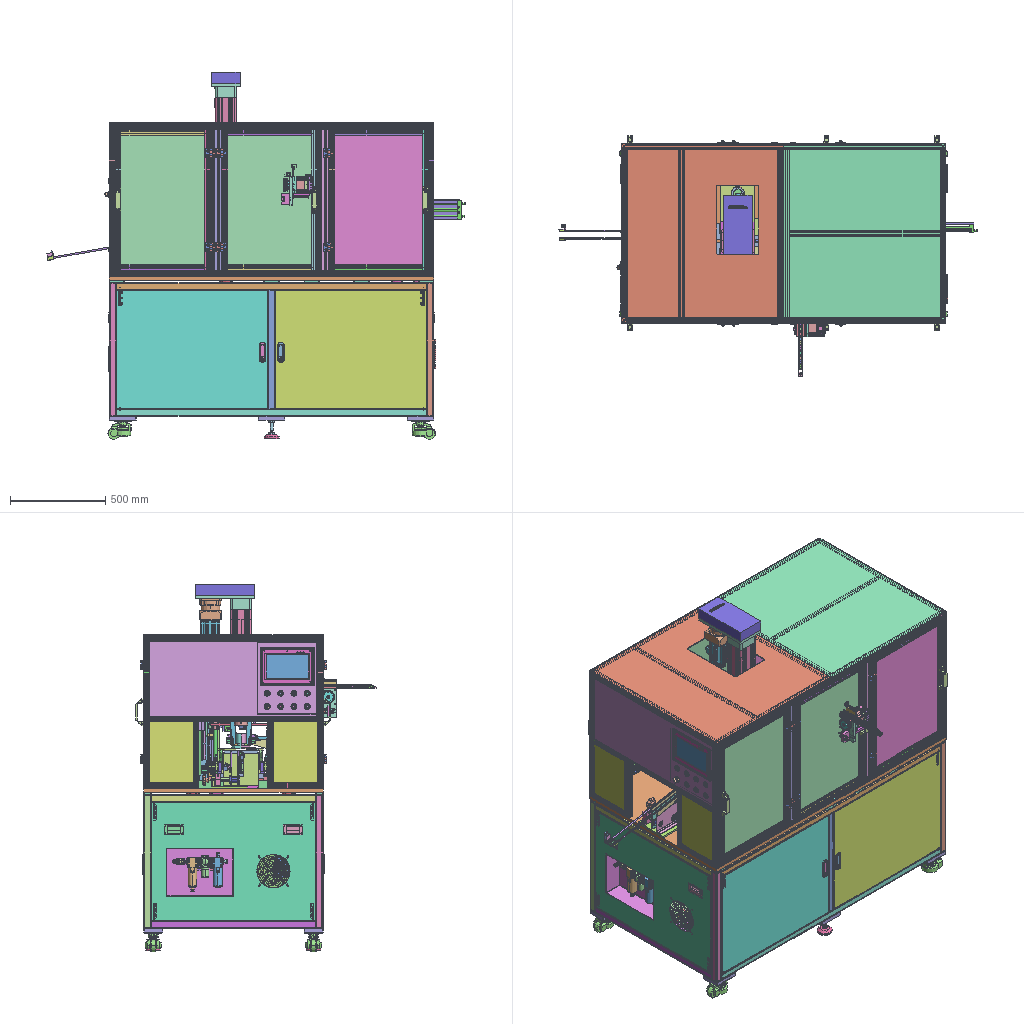Assembly | STEP file | 346 different items | 604 placed | box 2191 x 1257 x 1923 mm
Parts list (item | name | quantity | parent item | size | volume), first 266 of 346 items:
1 | 001-001-Profile frame_default<machined> | x1 | in 001-001-Machine frame_MV-FW80D | 1700 x 940 x 700 mm | 7004652 mm3
2 | 001-001-Small mounting plate | x10 | in 001-001-Machine frame_MV-FW80D | 80 x 40 x 12 mm | 38184 mm3
3 | 001-001-Main load plate | x1 | in 001-001-Machine frame_MV-FW80D | 1700 x 940 x 20 mm | 31960000 mm3
4 | 001-001-Foma caster mounting plate | x6 | in 001-001-Machine frame_MV-FW80D | 140 x 100 x 20 mm | 279640 mm3
5 | 001-001-hcaaa-d80-nj | x4 | in 001-001-Machine frame_MV-FW80D | 90 x 102 x 122.5 mm | 382378 mm3
6 | - | x2 | in 001-001-Machine frame_MV-FW80D | 78 x 134 x 78 mm | 111485 mm3
7 | 001-001-Machine frame door panel | x1 | in 001-001-Machine frame_MV-FW80D | 795 x 624 x 20 mm | 869592 mm3
8 | 001-001-hfy44-96-r | x1 | in 001-001-Machine frame_MV-FW80D | 18 x 22 x 96 mm | 10397 mm3
9 | 001-001-Fixed pin | x1 | in 001-001-Machine frame_MV-FW80D | 8 x 8 x 14 mm | 439.823 mm3
10 | 001-001-xax22-a106 | x1 | in 001-001-Machine frame_MV-FW80D | 69.5 x 40 x 106 mm | 52020 mm3
11 | 001-001- Mirror xax22-a106 | x2 | in 001-001-Machine frame_MV-FW80D | 69.5 x 40 x 106 mm | 52020 mm3
12 | 001-001-Mirror door panel | x2 | in 001-001-Machine frame_MV-FW80D | 795 x 624 x 20 mm | 869592 mm3
13 | 001-001-Mirror fixed pin | x2 | in 001-001-Machine frame_MV-FW80D | 8 x 8 x 14 mm | 439.823 mm3
14 | 001-001- Mirror hfy44-96-r | x3 | in 001-001-Machine frame_MV-FW80D | 18 x 22 x 96 mm | 10397 mm3
15 | 001-001- Mirror Mirror xax22-a106 | x1 | in 001-001-Machine frame_MV-FW80D | 69.5 x 40 x 106 mm | 52020 mm3
16 | 001-001-Mirror Mirror door panel | x1 | in 001-001-Machine frame_MV-FW80D | 795 x 624 x 20 mm | 869592 mm3
17 | 001-001-Mirror Mirror fixed pin | x1 | in 001-001-Machine frame_MV-FW80D | 8 x 8 x 14 mm | 439.823 mm3
18 | 001-001- Mirror Mirror hfy44-96-r | x3 | in 001-001-Machine frame_MV-FW80D | 18 x 22 x 96 mm | 10397 mm3
19 | 001-001-Machine frame end plate | x1 | in 001-001-Machine frame_MV-FW80D | 618 x 858 x 20 mm | 819319 mm3
20 | 001-001- Mirror Mirror Mirror hfy44-96-r | x1 | in 001-001-Machine frame_MV-FW80D | 18 x 22 x 96 mm | 10397 mm3
21 | 001-001-xad51-a100 | x1 | in 001-001-Machine frame_MV-FW80D | 54 x 20.5 x 100 mm | 9020 mm3
22 | 001-001- Mirror xad51-a100 | x1 | in 001-001-Machine frame_MV-FW80D | 54 x 20.5 x 100 mm | 9020 mm3
23 | FKL6622 cabinet fan and filter[FKL6622.230]_filter | x1 | in 001-001-FKL6622 cabinet fan and filter[FKL6622.230]_FKL6622.230 | 24.5 x 148.5 x 148.5 mm | 148645 mm3
24 | FKL6622 cabinet fan and filter[FKL6622.230]_120_G8025HA1S | x1 | in 001-001-FKL6622 cabinet fan and filter[FKL6622.230]_FKL6622.230 | 42.957 x 119.523 x 119.5 mm | 164726 mm3
25 | FKL6622 cabinet fan and filter[FKL6622.230]_TX120 | x1 | in 001-001-FKL6622 cabinet fan and filter[FKL6622.230]_FKL6622.230 | 116 x 5 x 116 mm | 5033 mm3
26 | 001-001-Mirror FKL6622 cabinet fan and filter[FKL6622.230]_filter | x1 | in 001-001-Mirror FKL6622 cabinet fan and filter[FKL6622.230] | 24.5 x 148.5 x 148.5 mm | 148645 mm3
27 | 001-001-Mirror FKL6622 cabinet fan and filter[FKL6622.230]_120_G8025HA1S | x1 | in 001-001-Mirror FKL6622 cabinet fan and filter[FKL6622.230] | 42.957 x 119.523 x 119.5 mm | 164726 mm3
28 | 001-001-Mirror FKL6622 cabinet fan and filter[FKL6622.230]_TX120 | x1 | in 001-001-Mirror FKL6622 cabinet fan and filter[FKL6622.230] | 116 x 5 x 116 mm | 5033 mm3
29 | - | x1 | in 001-001-Machine frame_MV-FW80D | 101.5 x 858 x 618 mm | 647667 mm3
30 | 001-001-Mirror Mirror Mirror hfy44-96-r | x2 | in 001-001-Machine frame_MV-FW80D | 18 x 22 x 96 mm | 10397 mm3
31 | 001-001-Mirrorxad51-a100 | x1 | in 001-001-Machine frame_MV-FW80D | 54 x 20.5 x 100 mm | 9020 mm3
32 | 001-001-Mirror Mirror hfy44-96-r | x1 | in 001-001-Machine frame_MV-FW80D | 18 x 22 x 96 mm | 10397 mm3
33 | 001-001-Mirror Mirror xad51-a100 | x1 | in 001-001-Machine frame_MV-FW80D | 54 x 20.5 x 100 mm | 9020 mm3
34 | 001-001-Mirror Mirror Mirror Mirror hfy44-96-r | x1 | in 001-001-Machine frame_MV-FW80D | 18 x 22 x 96 mm | 10397 mm3
35 | PH1002 | x1 | in 001-001-Air source treatment unit | 39.583 x 28.95 x 18 mm | 7378 mm3
36 | POC1002D | x1 | in 001-001-Air source treatment unit | 17 x 29 x 17 mm | 3444 mm3
37 | GAC30008S | x1 | in 001-001-Air source treatment unit | 195 x 203 x 83 mm | 926577 mm3
38 | HSV10 | x1 | in 001-001-Air source treatment unit | 35.5 x 35.5 x 68.5 mm | 34572 mm3
39 | 001-001-TX180 metal mesh cover[TX180]_TX180 | x1 | in 001-001-Machine frame_MV-FW80D | 175 x 5 x 175 mm | 9660 mm3
40 | 001-001-Machine frame bottom end plate | x2 | in 001-001-Machine frame_MV-FW80D | 788 x 858 x 20 mm | 1465006 mm3
41 | 200M10F | x1 | in 001-001-Valve island assembly | 60 x 24 x 251 mm | 220030 mm3
42 | BSL02 | x3 | in 001-001-Valve island assembly | 17.321 x 30 x 15 mm | 3652 mm3
43 | PC802 | x3 | in 001-001-Valve island assembly | 16.166 x 27 x 14 mm | 2706 mm3
44 | 4V21006B | x10 | in 001-001-Valve island assembly | 22 x 66.8 x 117.8 mm | 101337 mm3
45 | 001-003-Storage mechanism base plate | x1 | in 001-003-Shaft storage mechanism | 370 x 250 x 20 mm | 1842340 mm3
46 | 001-003-Storage mechanism vertical plate | x1 | in 001-003-Shaft storage mechanism | 250 x 550 x 15 mm | 1550347 mm3
47 | 001-003-Storage mechanism rib plate | x2 | in 001-003-Shaft storage mechanism | 110 x 546 x 15 mm | 610650 mm3
48 | - | x1 | - | 20 x 20 x 472 mm | 136774 mm3
49 | - | x1 | - | 44 x 58 x 42 mm | 39340 mm3
50 | 001-003-BK15 | x1 | in 001-003-Shaft storage mechanism | 70 x 48 x 39 mm | 76186 mm3
51 | 001-003-BF15 | x1 | in 001-003-Shaft storage mechanism | 70 x 48 x 20 mm | 44239 mm3
52 | 001-003-Shaft retaining ring 15-1 | x1 | in 001-003-Shaft storage mechanism | 16.7 x 18.72 x 1 mm | 79.464 mm3
53 | 001-003-Shaft storage motor mounting plate | x1 | in 001-003-Shaft storage mechanism | 210 x 71 x 15 mm | 181898 mm3
54 | 001-003-MSMF042L1D2 | x1 | in 001-003-Shaft storage mechanism | 165.5 x 143.937 x 60 mm | 465510 mm3
55 | 001-003-C-SCPS46-12-14 | x1 | in 001-003-Shaft storage mechanism | 29.8 x 46 x 46 mm | 36563 mm3
56 | - | x2 | - | 48 x 34.4 x 96 mm | 105086 mm3
57 | - | x2 | - | 23 x 22 x 480 mm | 205813 mm3
58 | 001-003-Shaft storage slider connecting plate | x1 | in 001-003-Shaft storage mechanism | 250 x 90 x 15 mm | 298680 mm3
59 | 001-003-Shaft storage magazine support plate | x1 | in 001-003-Shaft storage mechanism | 250 x 326 x 15 mm | 922956 mm3
60 | 001-003-Shaft storage magazine rib plate | x2 | in 001-003-Shaft storage mechanism | 55 x 170 x 15 mm | 86250 mm3
61 | 001-003-Shaft storage magazine base plate | x1 | in 001-003-Shaft storage mechanism | 288 x 190 x 10 mm | 533600 mm3
62 | 001-003-Shaft storage magazine side plate | x2 | in 001-003-Shaft storage mechanism | 288 x 210 x 10 mm | 591209 mm3
63 | 001-003-Shaft storage magazine rear plate | x1 | in 001-003-Shaft storage mechanism | 170 x 210 x 10 mm | 357000 mm3
64 | 001-003-Shaft storage magazine adjusting plate | x1 | in 001-003-Shaft storage mechanism | 270 x 203 x 10 mm | 530707 mm3
65 | 001-003-LJL74-d14 | x1 | in 001-003-Shaft storage mechanism | 45 x 45 x 30 mm | 14037 mm3
66 | 001-003-LHC07-D14-L241-S16 | x1 | in 001-003-Shaft storage mechanism | 14 x 14 x 241 mm | 32328 mm3
67 | 001-003-LHF04-R10, | x1 | in 001-003-Shaft storage mechanism | 14 x 52 x 42 mm | 14223 mm3
68 | 001-003-LHF08-Q10, | x1 | in 001-003-Shaft storage mechanism | 43.5 x 64.4 x 76.26 mm | 63450 mm3
69 | 001-003-HAK13-D60-M8 | x1 | in 001-003-Shaft storage mechanism | 60 x 32 x 57.857 mm | 42793 mm3
70 | 001-003-Feeding plate | x1 | in 001-003-Shaft storage mechanism | 170 x 335 x 8 mm | 427857 mm3
71 | 001-003-Shaft storage cylinder mounting plate | x1 | in 001-003-Shaft storage mechanism | 190 x 410.5 x 10 mm | 720796 mm3
72 | 001-003-Shaft storage support plate reinforcing rib | x2 | in 001-003-Shaft storage mechanism | 28 x 60 x 10 mm | 7819 mm3
73 | 001-003-ACQS_32x200_B_P_b | x1 | - | 250.5 x 49.5 x 45 mm | 256308 mm3
74 | - | x1 | - | 271.5 x 32 x 32 mm | 65744 mm3
75 | 001-003-ACQ_32_Nut | x1 | - | 8 x 21.939 x 19 mm | 1486 mm3
76 | 001-003-CMSG_GN | x2 | - | 40.5 x 5.8 x 4.4 mm | 628.814 mm3
77 | 001-003-Shaft storage cylinder mounting seat | x1 | in 001-003-Shaft storage mechanism | 78 x 45 x 20 mm | 40773 mm3
78 | 001-003-PH601 | x2 | in 001-003-Shaft storage mechanism | 29.851 x 25 x 13.702 mm | 3817 mm3
79 | 001-003-F-M14X150F, | x1 | in 001-003-Shaft storage mechanism | 34.5 x 34.5 x 70 mm | 35671 mm3
80 | 001-003-Shaft storage cylinder connection block | x1 | in 001-003-Shaft storage mechanism | 36 x 45 x 20 mm | 18557 mm3
81 | 001-003-GBC26_D13 | x2 | in 001-003-Shaft storage mechanism | 27 x 42 x 26 mm | 11275 mm3
82 | 001-003-SCD21_D13_L330_M5 | x2 | in 001-003-Shaft storage mechanism | 13 x 13 x 330 mm | 43651 mm3
83 | 001-003-LMW56_d13 | x2 | in 001-003-Shaft storage mechanism | 51 x 30 x 75 mm | 69103 mm3
84 | 001-003-E_LME13_d16 | x2 | in 001-003-Shaft storage mechanism | 37 x 48 x 48 mm | 18897 mm3
85 | 001-003-SCJ22_D16_L170_M5_N5 | x2 | in 001-003-Shaft storage mechanism | 16 x 16 x 170 mm | 33866 mm3
86 | 001-004-Feeding mechanism feed base plate | x1 | in 001-004-Feeding mechanism | 460 x 95 x 10 mm | 433460 mm3
87 | - | x1 | - | 459 x 101.4 x 39 mm | 391134 mm3
88 | _CMSG_ | x2 | - | 40.5 x 5.8 x 4.4 mm | 628.814 mm3
89 | - | x1 | - | 75 x 92 x 38 mm | 179586 mm3
90 | 001-004-Feeding mechanism adapter plate | x1 | in 001-004-Feeding mechanism | 75 x 120 x 12 mm | 78391 mm3
91 | 001-004-Feeding mechanism fixing plate | x1 | in 001-004-Feeding mechanism | 75 x 95 x 10 mm | 69450 mm3
92 | 001-004-Feeding mechanism reinforcing rib | x1 | in 001-004-Feeding mechanism | 40 x 60 x 15 mm | 13822 mm3
93 | 001-004-Feeding mechanism push block | x1 | in 001-004-Feeding mechanism | 55 x 80 x 50 mm | 193083 mm3
94 | 001-004-RCJ11_D30 | x2 | in 001-004-Feeding mechanism | 60 x 60 x 90 mm | 153329 mm3
95 | 001-004-SCD11_D30_L598_M6 | x2 | in 001-004-Feeding mechanism | 598 x 30 x 30 mm | 422409 mm3
96 | 001-004-GAY12_D30 | x2 | in 001-004-Feeding mechanism | 79 x 57 x 42 mm | 84373 mm3
97 | 001-004-Feeding mechanism shaft slideway base plate | x1 | in 001-004-Feeding mechanism | 200 x 180 x 10 mm | 352263 mm3
98 | 001-004-Feeding mechanism shaft slideway rear plate | x1 | in 001-004-Feeding mechanism | 380 x 102.993 x 10 mm | 333174 mm3
99 | 001-004-Feeding mechanism shaft slideway vertical plate | x1 | in 001-004-Feeding mechanism | 200 x 100 x 10 mm | 181569 mm3
100 | 001-004-Feeding mechanism shaft slideway side plate | x2 | in 001-004-Feeding mechanism | 170 x 90 x 10 mm | 116972 mm3
101 | 001-004-Feeding mechanism shaft slideway cover plate | x1 | in 001-004-Feeding mechanism | 170 x 52.886 x 200 mm | 357000 mm3
102 | 001-004-Feeding mechanism feed guide chute 1 | x1 | in 001-004-Feeding mechanism | 90 x 13.679 x 177.909 mm | 23460 mm3
103 | 001-004-Feeding mechanism feed guide chute 2 | x1 | in 001-004-Feeding mechanism | 32 x 13.679 x 180.909 mm | 10329 mm3
104 | 001-004-Feeding mechanism proximity switch mounting sheet metal | x2 | in 001-004-Feeding mechanism | 48 x 35.5 x 20 mm | 2128 mm3
105 | 001-004-TE-12N4C, _TE-12N4C | x2 | in 001-004-Feeding mechanism | 18 x 20.785 x 88.5 mm | 9092 mm3
106 | 001-004-12PB125UBody | x1 | - | 179 x 15 x 15 mm | 9809 mm3
107 | 001-004-12PB125URod | x1 | - | 182.85 x 11.5 x 11.5 mm | 4627 mm3
108 | 001-004-PB12nut | x1 | - | 4 x 16.166 x 14 mm | 434.114 mm3
109 | 001-004-124nut1 | x1 | - | 4 x 9.238 x 8 mm | 164.287 mm3
110 | - | x2 | - | 37.5 x 24.7 x 16 mm | 1895 mm3
111 | 001-004-Feeding mechanism cylinder mounting seat | x1 | in 001-004-Feeding mechanism | 24 x 46 x 29 mm | 6337 mm3
112 | - | x1 | - | 20 x 8 x 28.991 mm | 3251 mm3
113 | - | x1 | - | 9 x 6.5 x 200 mm | 10020 mm3
114 | 001-004-Feeding mechanism slider connecting plate | x1 | in 001-004-Feeding mechanism | 48 x 35 x 26 mm | 20800 mm3
115 | 001-004-F_M5X080U | x1 | in 001-004-Feeding mechanism | 18 x 10 x 36 mm | 2763 mm3
116 | 001-004-TBH02_d5_L20 | x1 | in 001-004-Feeding mechanism | 29.5 x 7.985 x 7.985 mm | 581.04 mm3
117 | 001-004-Feeding mechanism push plate | x1 | in 001-004-Feeding mechanism | 18 x 130 x 4 mm | 9329 mm3
118 | 001-004-Feeding mechanism hydraulic buffer mounting plate | x1 | in 001-004-Feeding mechanism | 25 x 40 x 12 mm | 11215 mm3
119 | ACA_1007_1_Body | x1 | in 001-004-ACA1007_1 | 10 x 63.5 x 10 mm | 4041 mm3
120 | ACA_1007_1_NT | x2 | in 001-004-ACA1007_1 | 14 x 4 x 15.686 mm | 394.078 mm3
121 | 001-004-Hexagon socket countersunk head screw M6x10 | x2 | in 001-004-Feeding mechanism | 11.3 x 10 x 11.3 mm | 345.405 mm3
122 | 001-004-Feeding mechanism shaft entry channel base plate | x2 | in 001-004-Feeding mechanism | 249 x 210 x 10 mm | 317210 mm3
123 | 001-004-Feeding mechanism support profile_default<machined> | x2 | in 001-004-Feeding mechanism | 151 x 30 x 30 mm | 50748 mm3
124 | 001-004-Feeding mechanism slide connecting plate | x1 | in 001-004-Feeding mechanism | 151 x 180 x 10 mm | 271800 mm3
125 | 001-004-Feeding mechanism shaft entry channel plate | x1 | in 001-004-Feeding mechanism | 230 x 198.5 x 10 mm | 116591 mm3
126 | 001-004-Feeding mechanism shaft entry channel baffle | x1 | in 001-004-Feeding mechanism | 10 x 210 x 10 mm | 21000 mm3
127 | Planar support platform panel | x1 | in 001-007-Planar support mechanism | 1430 x 180 x 15 mm | 3191288 mm3
128 | Planar support platform vertical plate | x2 | in 001-007-Planar support mechanism | 180 x 170 x 15 mm | 404827 mm3
129 | Planar support platform base | x2 | in 001-007-Planar support mechanism | 80 x 180 x 15 mm | 210480 mm3
130 | Planar support spacer block | x1 | in 001-007-Planar support mechanism | 30 x 60 x 10 mm | 17805 mm3
131 | Planar support stopper | x1 | in 001-007-Planar support mechanism | 120 x 74.54 x 5 mm | 21231 mm3
132 | 001-005-Shaft threading fixture base plate | x1 | in 001-005-Shaft threading fixture mechanism | 120 x 90 x 12 mm | 127352 mm3
133 | 001-005-Shaft threading fixture vertical plate | x1 | in 001-005-Shaft threading fixture mechanism | 90 x 310 x 12 mm | 332004 mm3
134 | 001-005-Shaft threading fixture rib plate | x2 | in 001-005-Shaft threading fixture mechanism | 80 x 300 x 10 mm | 142000 mm3
135 | 001-005-Shaft threading fixture adapter plate | x1 | in 001-005-Shaft threading fixture mechanism | 90 x 142 x 15 mm | 177188 mm3
136 | 001-005-Shaft threading fixture reinforcing rib | x1 | in 001-005-Shaft threading fixture mechanism | 120 x 45 x 15 mm | 55125 mm3
137 | 001-005-Shaft threading fixture cylinder mounting plate | x1 | in 001-005-Shaft threading fixture mechanism | 142 x 130 x 12 mm | 162627 mm3
138 | - | x1 | in 001-005-HFD16X60_OP_ | 56 x 147 x 32.5 mm | 222533 mm3
139 | - | x2 | in 001-005-HFD16X60_OP_ | 21.8 x 40 x 14 mm | 9965 mm3
140 | 001-005-PSL6M5AD_S | x2 | in 001-005-Shaft threading fixture mechanism | 28.5 x 30 x 12.5 mm | 2577 mm3
141 | 001-005-Shaft threading fixture adapter gripper | x1 | in 001-005-Shaft threading fixture mechanism | 48 x 121.5 x 12 mm | 37787 mm3
142 | 001-005-Shaft threading fixture mould | x1 | in 001-005-Shaft threading fixture mechanism | 48 x 70 x 77 mm | 85963 mm3
143 | 001-005-Mirror Mould | x1 | in 001-005-Shaft threading fixture mechanism | 48 x 70 x 77 mm | 85963 mm3
144 | 001-005-Mirror adapter gripper | x1 | in 001-005-Shaft threading fixture mechanism | 48 x 121.5 x 12 mm | 37787 mm3
145 | 001-005-PCB01_5_H6 | x1 | in 001-005-Shaft threading fixture mechanism | 9 x 12 x 32 mm | 2450 mm3
146 | 001-005-PAZ32_M5_L20 | x1 | in 001-005-Shaft threading fixture mechanism | 15 x 15 x 49.6 mm | 3017 mm3
147 | 001-006-Pre-insertion mechanism pressure plate | x1 | in 001-006-Pre-insertion mechanism | 400 x 70 x 12 mm | 298236 mm3
148 | 001-006-ACQS_16x3030_b | x1 | in 001-006-ACQ16x30SBLB_0_CMSG2_ | 60.5 x 29 x 29 mm | 34569 mm3
149 | 001-006-ACQS_16x30_B_30r | x1 | in 001-006-ACQ16x30SBLB_0_CMSG2_ | 72 x 16 x 16 mm | 5884 mm3
150 | 001-006-ACQ_16_Nut | x1 | in 001-006-ACQ16x30SBLB_0_CMSG2_ | 5 x 11.547 x 10 mm | 329.448 mm3
151 | 001-006-F_ACQ16LB | x2 | in 001-006-ACQ16x30SBLB_0_CMSG2_ | 13 x 33.5 x 48 mm | 3042 mm3
152 | - | x4 | in 001-006-ACQ16x30SBLB_0_CMSG2_ | 16 x 7 x 7 mm | 285.452 mm3
153 | 001-006-CMSG_GN | x4 | in 001-006-ACQ16x30SBLB_0_CMSG2_ | 40.5 x 5.8 x 4.4 mm | 628.814 mm3
154 | 001-006-Rail_MGN9R00801HM_7_5 | x1 | in 001-006-MGN9C1R0080Z0HM_No_Set_E1_7_5 | 80 x 6.5 x 9 mm | 3913 mm3
155 | MGN9CZ0HM | x1 | in 001-006-Pre-insertion mechanism slider | 26.9 x 8 x 20 mm | 3027 mm3
156 | EndSeal_MGN9 | x2 | in 001-006-Pre-insertion mechanism slider | 1 x 7.7 x 19.6 mm | 85.449 mm3
157 | Bolt_MG9 | x4 | in 001-006-Pre-insertion mechanism slider | 4 x 3 x 3 mm | 10.872 mm3
158 | MG_P_Screw_9_N | x1 | in 001-006-Pre-insertion mechanism slider | 1.333 x 4.5 x 1.333 mm | 5.111 mm3
159 | MG_Plug_Screw_9_N | x1 | in 001-006-Pre-insertion mechanism slider | 1.333 x 4.5 x 1.333 mm | 5.052 mm3
160 | 001-006-MirrorRail_MGN9R00801HM_7_5 | x1 | in 001-006-MirrorMGN9C1R0080Z0HM_No_Set_E1_7_5 | 80 x 6.5 x 9 mm | 3913 mm3
161 | 001-006-MirrorMGN9CZ0HM | x1 | in 001-006-Mirror slider | 26.9 x 8 x 20 mm | 3027 mm3
162 | 001-006-MirrorEndSeal_MGN9 | x2 | in 001-006-Mirror slider | 1 x 7.7 x 19.6 mm | 85.449 mm3
163 | 001-006-MirrorBolt_MG9 | x4 | in 001-006-Mirror slider | 4 x 3 x 3 mm | 10.872 mm3
164 | 001-006-MirrorMG_P_Screw_9_N | x1 | in 001-006-Mirror slider | 1.333 x 4.5 x 1.333 mm | 5.111 mm3
165 | 001-006-MirrorMG_Plug_Screw_9_N | x1 | in 001-006-Mirror slider | 1.333 x 4.5 x 1.333 mm | 5.052 mm3
166 | 001-006-Pre-insertion mechanism slider connecting plate | x1 | in 001-006-Pre-insertion mechanism | 64 x 35 x 4 mm | 8840 mm3
167 | 001-006-F_M6X100U | x1 | in 001-006-Pre-insertion mechanism | 20 x 11 x 40 mm | 3632 mm3
168 | 001-006-TBH02_d6_L10 | x1 | in 001-006-Pre-insertion mechanism | 21 x 8.981 x 8.981 mm | 576.249 mm3
169 | 001-006-TAC01_M8_L55 | x1 | in 001-006-Pre-insertion mechanism | 13 x 13 x 63 mm | 3670 mm3
170 | 001-006-TBK31_M8 | x1 | in 001-006-Pre-insertion mechanism | 7.5 x 15.011 x 13 mm | 822.445 mm3
171 | 001-006-PBP10_M6_H11 | x1 | in 001-006-Pre-insertion mechanism | 9 x 16 x 30 mm | 3306 mm3
172 | 001-006-TAC01_M6_L50 | x1 | in 001-006-Pre-insertion mechanism | 10 x 10 x 56 mm | 1803 mm3
173 | 001-006-TBK52_M6 | x1 | in 001-006-Pre-insertion mechanism | 5 x 11.547 x 10 mm | 332.113 mm3
174 | 001-006-SDAJS_20x60_60b | x1 | - | 92.5 x 36 x 34 mm | 63819 mm3
175 | 001-006-SDAJS_20x60_B2060_r | x1 | - | 212.5 x 19.9 x 19.9 mm | 13647 mm3
176 | - | x1 | - | 5 x 11.547 x 10 mm | 329.448 mm3
177 | - | x1 | - | 36 x 15 x 15 mm | 4516 mm3
178 | - | x1 | - | 5 x 11.547 x 10 mm | 329.448 mm3
179 | 001-006-PSL6M5AD_S | x4 | in 001-006-Pre-insertion mechanism | 28.5 x 30 x 12.5 mm | 2577 mm3
180 | 001-006-SAD21_D20_L430 | x2 | in 001-006-Pre-insertion mechanism | 430 x 20 x 20 mm | 135028 mm3
181 | 001-006-LME13_d20 | x2 | in 001-006-Pre-insertion mechanism | 54 x 54 x 42 mm | 26442 mm3
182 | _GAY12-D20-001.stp | x2 | in GAY12-D20.stp | 64 x 42 x 34 mm | 29366 mm3
183 | _GAY12-D20-002.stp | x2 | in GAY12-D20.stp | 39.787 x 19.4 x 23 mm | 7951 mm3
184 | _GAY01-D20-003_2.stp | x8 | in GAY12-D20.stp | 9 x 9 x 25 mm | 670.975 mm3
185 | 001-006-Pre-insertion mechanism buffer mounting plate | x1 | in 001-006-Pre-insertion mechanism | 80 x 30 x 12 mm | 22818 mm3
186 | 001-006-F-M6X100F | x1 | in 001-006-Pre-insertion mechanism | 34.5 x 14.8 x 14 mm | 3454 mm3
187 | _ACA-1007-1_Body.stp | x1 | in ACA1007-1.stp | 10 x 63.5 x 10 mm | 4041 mm3
188 | _ACA-1007-1_NT.stp | x2 | in ACA1007-1.stp | 14 x 4 x 15.686 mm | 394.083 mm3
189 | _VED02-F15-001.stp | x1 | in VBD02-F15-R28-N20.stp | 25 x 19.468 x 39.663 mm | 3938 mm3
190 | _VBD02-F15-R28-N20-001.stp | x20 | in VBD02-F15-R28-N20.stp | 25.1 x 19.5 x 44.39 mm | 5553 mm3
191 | _VED02-F15-002.stp | x1 | in VBD02-F15-R28-N20.stp | 25 x 19.467 x 39.663 mm | 5123 mm3
192 | 001-006-Pre-insertion mechanism drag chain mounting plate | x1 | in 001-006-Pre-insertion mechanism | 60 x 68 x 3 mm | 8197 mm3
193 | 001-006-Pre-insertion mechanism drag chain mounting plate 2 | x1 | in 001-006-Pre-insertion mechanism | 30 x 37 x 30 mm | 5591 mm3
194 | 001-008-Traverse module base plate | x1 | in 001-008-Traverse module | 549.5 x 160 x 15 mm | 1271693 mm3
195 | - | x1 | - | 15 x 15 x 523 mm | 87491 mm3
196 | - | x1 | - | 40 x 48 x 47 mm | 29180 mm3
197 | 001-008-LEF01-d12-F60S-h25 | x1 | in 001-008-Traverse module | 70 x 60 x 83.5 mm | 110903 mm3
198 | 001-008-LEB51-12 | x1 | in 001-008-Traverse module | 20 x 43 x 70 mm | 40674 mm3
199 | MSMF022LNoStraight_b | x1 | in 001-008-MSMF022L1C2 | 109.5 x 60 x 60 mm | 260570 mm3
200 | Cable_Motor_Bottom_03_CM2_MSMF | x1 | in 001-008-MSMF022L1C2 | 45.598 x 29.85 x 36 mm | 13881 mm3
201 | Cable_Motor_Top_03_MSMF | x1 | in 001-008-MSMF022L1C2 | 7.8 x 34.633 x 7.8 mm | 896.959 mm3
202 | Motor_Connector_2 | x1 | in 001-008-MSMF022L1C2 | 23.7 x 14.55 x 11.2 mm | 1255 mm3
203 | Cable_Brake_Top_03_CE02_MSMF | x1 | in 001-008-MSMF022L1C2 | 27.962 x 30.887 x 22.9 mm | 4595 mm3
204 | Cable_Brake_Top_03_CE01_MSMF | x1 | in 001-008-MSMF022L1C2 | 6 x 28.381 x 6 mm | 414.888 mm3
205 | MHMF_Connector_9_Pin_A6 | x1 | in 001-008-MSMF022L1C2 | 23.7 x 19 x 14.5 mm | 1788 mm3
206 | 001-008-DBA61-D32-d10-e11 | x1 | in 001-008-Traverse module | 41 x 32 x 32 mm | 22290 mm3
207 | 001-008-Rail_HGR15R04801_20_0 | x2 | in 001-008-HGH15CA1R0480Z0H_No_Set_E1_20_0 | 480 x 15 x 15 mm | 88626 mm3
208 | Block_HGH15CAZ0C | x4 | in 001-008-Traverse module slider | 55.4 x 23.7 x 34 mm | 33117 mm3
209 | 920019A1 | x8 | in 001-008-Traverse module slider | 3 x 18.7 x 32.4 mm | 1294 mm3
210 | HG15_34310002 | x4 | in 001-008-Traverse module slider | 5 x 12.3 x 5.774 mm | 186.95 mm3
211 | Bolt_HG15 | x16 | in 001-008-Traverse module slider | 11.88 x 5.5 x 5.5 mm | 74.446 mm3
212 | HG15_PlugScrew | x4 | in 001-008-Traverse module slider | 4.324 x 7.5 x 4.324 mm | 90.944 mm3
213 | 001-008-Traverse module nut seat | x1 | in 001-008-Traverse module | 40 x 70 x 39 mm | 82202 mm3
214 | 001-008-Traverse module slider connecting plate | x1 | in 001-008-Traverse module | 340 x 180 x 25 mm | 1323417 mm3
215 | 001-008-SENAM33H-500-V10-W250-X490 | x1 | in 001-008-Traverse module | 500 x 9 x 6 mm | 15737 mm3
216 | 001-008-PM-F25 (Panasonic) | x3 | in 001-008-Traverse module | 15.4 x 12 x 11.7 mm | 857.476 mm3
217 | 001-008-Traverse module detection sheet metal | x1 | in 001-008-Traverse module | 27 x 20 x 70 mm | 6118 mm3
218 | 001-008-_SDAJS-25x30_30b | x1 | in 001-008-SDAJ25x30-10SB_0x0_+_CMSG-2_ | 65 x 42 x 40 mm | 54492 mm3
219 | 001-008-_SDAJS-25x30-B1030_r | x1 | in 001-008-SDAJ25x30-10SB_0x0_+_CMSG-2_ | 151 x 24.9 x 24.9 mm | 17310 mm3
220 | 001-008-_SDAJ-25- M8x1.25 | x1 | in 001-008-SDAJ25x30-10SB_0x0_+_CMSG-2_ | 6 x 13.856 x 12 mm | 523.34 mm3
221 | 001-008-_SDA-25-M8x1.2510 - A_Nut | x1 | in 001-008-SDAJ25x30-10SB_0x0_+_CMSG-2_ | 29 x 20 x 20 mm | 6775 mm3
222 | 001-008-_SDAJ-25- M8x1.25SDAJ_NUT | x1 | in 001-008-SDAJ25x30-10SB_0x0_+_CMSG-2_ | 6 x 13.856 x 12 mm | 523.34 mm3
223 | 001-008-_CMSG_GN | x2 | in 001-008-SDAJ25x30-10SB_0x0_+_CMSG-2_ | 40.5 x 5.8 x 4.4 mm | 628.814 mm3
224 | 001-008-WIB01-25-H35-N5 | x1 | in 001-008-Traverse module | 42 x 55 x 22 mm | 19975 mm3
225 | - | x4 | - | 34 x 23.6 x 65.8 mm | 37815 mm3
226 | - | x2 | - | 15 x 15 x 300 mm | 59817 mm3
227 | 001-008-Traverse module gripper mounting plate | x1 | in 001-008-Traverse module | 180 x 50 x 18 mm | 146550 mm3
228 | 001-008-F-M8X125F | x1 | in 001-008-Traverse module | 24 x 24 x 51 mm | 10568 mm3
229 | 001-008-Traverse module transfer vertical plate | x1 | in 001-008-Traverse module | 600 x 111 x 15 mm | 459001 mm3
230 | 001-008-PSL6M5A-S | x2 | in 001-008-Traverse module | 28.5 x 30 x 12.5 mm | 2577 mm3
231 | 001-008-Traverse module reinforcing rib | x3 | in 001-008-Traverse module | 45 x 60 x 15 mm | 17464 mm3
232 | 001-008-Traverse module transfer fixture | x1 | in 001-008-Traverse module | 950 x 90 x 10 mm | 745703 mm3
233 | 001-008-MirrorPSL6M5A-S | x2 | in 001-008-Traverse module | 28.5 x 30 x 12.5 mm | 2578 mm3
234 | 001-008-Mirror_SDAJS-25x30_30b | x1 | in 001-008-MirrorSDAJ25x30-10SB_0x0_+_CMSG-2_ | 65 x 42 x 40 mm | 54492 mm3
235 | 001-008-Mirror_SDAJS-25x30-B1030_r | x1 | in 001-008-MirrorSDAJ25x30-10SB_0x0_+_CMSG-2_ | 151 x 24.9 x 24.9 mm | 17310 mm3
236 | 001-008-Mirror_SDAJ-25- M8x1.25 | x1 | in 001-008-MirrorSDAJ25x30-10SB_0x0_+_CMSG-2_ | 6 x 13.856 x 12 mm | 523.506 mm3
237 | 001-008-Mirror_SDA-25-M8x1.2510 - A_Nut | x1 | in 001-008-MirrorSDAJ25x30-10SB_0x0_+_CMSG-2_ | 29 x 20 x 20 mm | 6778 mm3
238 | 001-008-Mirror_SDAJ-25- M8x1.25SDAJ_NUT | x1 | in 001-008-MirrorSDAJ25x30-10SB_0x0_+_CMSG-2_ | 6 x 13.856 x 12 mm | 523.506 mm3
239 | 001-008-Mirror_CMSG_GN | x2 | in 001-008-MirrorSDAJ25x30-10SB_0x0_+_CMSG-2_ | 40.5 x 5.8 x 4.4 mm | 628.814 mm3
240 | 001-008-MirrorWIB01-25-H35-N5 | x1 | in 001-008-Traverse module | 42 x 55 x 22 mm | 19975 mm3
241 | 001-008-MirrorF-M8X125F | x1 | in 001-008-Traverse module | 24 x 24 x 51 mm | 10568 mm3
242 | 001-008-Mirror transfer vertical plate | x1 | in 001-008-Traverse module | 600 x 111 x 15 mm | 459001 mm3
243 | 001-008-Mirror reinforcing rib | x3 | in 001-008-Traverse module | 45 x 60 x 15 mm | 17464 mm3
244 | 001-008-Mirror gripper mounting plate | x1 | in 001-008-Traverse module | 180 x 50 x 18 mm | 146550 mm3
245 | 001-008-Mirror transfer fixture | x1 | in 001-008-Traverse module | 950 x 90 x 10 mm | 745703 mm3
246 | 001-010-Waste base plate | x1 | in 001-010-Waste mechanism | 650 x 90 x 12 mm | 699774 mm3
247 | 001-010-Mounting vertical plate | x1 | in 001-010-Waste mechanism | 650 x 150 x 15 mm | 1380441 mm3
248 | 001-010-Waste reinforcing rib plate | x2 | in 001-010-Waste mechanism | 90 x 50 x 15 mm | 42376 mm3
249 | 001-010-Waste column profile_default<machined> | x1 | in 001-010-Waste mechanism | 425 x 90 x 90 mm | 830601 mm3
250 | 001-010-ABC01-4510-50-80 | x2 | in 001-010-Waste mechanism | 50 x 50 x 80 mm | 63404 mm3
251 | 001-010-ABC01-4510-90-80 | x2 | in 001-010-Waste mechanism | 90 x 90 x 80 mm | 146220 mm3
252 | 001-010-Waste through-beam photoelectric mounting plate | x1 | in 001-010-Waste mechanism | 38 x 193 x 110 mm | 56258 mm3
253 | 001-010-Through-beam photoelectric sensor (Delta) | x2 | in 001-010-Waste mechanism | - | -
254 | 001-010-Leadshine 86CME45 (closed loop) | x1 | in 001-010-Waste mechanism | 86 x 97.458 x 148.7 mm | 429734 mm3
255 | 001-010-EBJ22-S5M150-40-B-N-d14 | x1 | in 001-010-Waste mechanism | 67 x 67 x 34 mm | 78726 mm3
256 | 001-010-ECC15-S5M150-40-E-d15 | x1 | in 001-010-Waste mechanism | 67 x 67 x 34 mm | 65778 mm3
257 | 001-010-ZS-FK15 | x1 | in 001-010-Waste mechanism | 63 x 63 x 43 mm | 52330 mm3
258 | 001-010-Waste driven wheel mounting shaft | x1 | in 001-010-Waste mechanism | 18 x 18 x 81 mm | 14775 mm3
259 | 001-010-Belt 1-56 | x1 | in 001-010-Waste mechanism | 635.7 x 68.7 x 15 mm | 40306 mm3
260 | - | x1 | - | 34 x 23.6 x 65.8 mm | 37815 mm3
261 | - | x1 | - | 15 x 15 x 540 mm | 107671 mm3
262 | 001-010-Waste slider connecting plate | x1 | in 001-010-Waste mechanism | 60 x 90 x 37.5 mm | 99990 mm3
263 | 001-010-ECY51-S5M-150 | x1 | in 001-010-Waste mechanism | 33 x 6 x 36 mm | 5925 mm3
264 | 001-010-Waste limit block | x2 | in 001-010-Waste mechanism | 56 x 43 x 15 mm | 34918 mm3
265 | 001-010-ACA1007-1 | x2 | in 001-010-Waste mechanism | 14 x 63.5 x 15.686 mm | 4829 mm3
266 | 001-010-TAC01-M6-L50 | x2 | in 001-010-Waste mechanism | 10 x 10 x 56 mm | 1803 mm3
Placements (level | parent | child | x y z in mm | rotation matrix by rows), first 181 of 671 lines:
1 | subassembly 2 | 001-001-Machine frame_MV-FW80D | -0.0 -0.0 -0.0 | 1 0 0 0 1 0 0 0 1
2 | 001-001-Machine frame_MV-FW80D | 001-001-Profile frame_default<machined> | -0.0 -0.0 -0.0 | 1 0 0 0 1 0 0 0 1
2 | 001-001-Machine frame_MV-FW80D | 001-001-Small mounting plate | 0.0 -0.0 680.0 | 1 0 0 0 1 0 0 0 1
2 | 001-001-Machine frame_MV-FW80D | 001-001-Small mounting plate | 810.0 -0.0 680.0 | 1 0 0 0 1 0 0 0 1
2 | 001-001-Machine frame_MV-FW80D | 001-001-Small mounting plate | 1620.0 -0.0 680.0 | 1 0 0 0 1 0 0 0 1
2 | 001-001-Machine frame_MV-FW80D | 001-001-Small mounting plate | 0.0 -900.0 680.0 | 1 0 0 0 1 0 0 0 1
2 | 001-001-Machine frame_MV-FW80D | 001-001-Small mounting plate | 810.0 -900.0 680.0 | 1 0 0 0 1 0 0 0 1
2 | 001-001-Machine frame_MV-FW80D | 001-001-Small mounting plate | 1620.0 -900.0 680.0 | 1 0 0 0 1 0 0 0 1
2 | 001-001-Machine frame_MV-FW80D | 001-001-Small mounting plate | 1280.0 -0.0 680.0 | 1 0 0 0 1 0 0 0 1
2 | 001-001-Machine frame_MV-FW80D | 001-001-Small mounting plate | 1280.0 -900.0 680.0 | 1 0 0 0 1 0 0 0 1
2 | 001-001-Machine frame_MV-FW80D | 001-001-Small mounting plate | 1020.0 -0.0 680.0 | 1 0 0 0 1 0 0 0 1
2 | 001-001-Machine frame_MV-FW80D | 001-001-Small mounting plate | 1020.0 -900.0 680.0 | 1 0 0 0 1 0 0 0 1
2 | 001-001-Machine frame_MV-FW80D | 001-001-Main load plate | -0.0 -0.0 692.0 | 1 0 0 0 1 0 0 0 1
2 | 001-001-Machine frame_MV-FW80D | 001-001-Foma caster mounting plate | 0.0 -0.0 -20.0 | -1 0 0 0 1 0 0 0 -1
2 | 001-001-Machine frame_MV-FW80D | 001-001-Foma caster mounting plate | 0.0 840.0 -20.0 | -1 0 0 0 1 0 0 0 -1
2 | 001-001-Machine frame_MV-FW80D | 001-001-Foma caster mounting plate | 780.0 -0.0 -20.0 | -1 0 0 0 1 0 0 0 -1
2 | 001-001-Machine frame_MV-FW80D | 001-001-Foma caster mounting plate | 780.0 840.0 -20.0 | -1 0 0 0 1 0 0 0 -1
2 | 001-001-Machine frame_MV-FW80D | 001-001-Foma caster mounting plate | 1560.0 -0.0 -20.0 | -1 0 0 0 1 0 0 0 -1
2 | 001-001-Machine frame_MV-FW80D | 001-001-Foma caster mounting plate | 1560.0 840.0 -20.0 | -1 0 0 0 1 0 0 0 -1
2 | 001-001-Machine frame_MV-FW80D | 001-001-hcaaa-d80-nj | 826.5 420.0 -111.0 | 0 0 1 1 0 0 0 1 0
2 | 001-001-Machine frame_MV-FW80D | 001-001-hcaaa-d80-nj | 826.5 -420.0 -111.0 | 0 0 1 1 0 0 0 1 0
2 | 001-001-Machine frame_MV-FW80D | 001-001-hcaaa-d80-nj | -826.5 420.0 -111.0 | 0 0 -1 -1 0 0 0 1 0
2 | 001-001-Machine frame_MV-FW80D | 001-001-hcaaa-d80-nj | -826.5 -420.0 -111.0 | 0 0 -1 -1 0 0 0 1 0
2 | 001-001-Machine frame_MV-FW80D | subassembly 3 | 0.0 420.0 -3.0 | 0.866 0 0.5 0.5 0 -0.866 0 1 -0
2 | 001-001-Machine frame_MV-FW80D | subassembly 3 | 0.0 -420.0 -3.0 | 0.866 0 -0.5 -0.5 0 -0.866 0 1 -0
2 | 001-001-Machine frame_MV-FW80D | 001-001-Machine frame door panel | -0.0 470.0 -0.0 | -1 0 0 0 0 1 0 1 0
2 | 001-001-Machine frame_MV-FW80D | 001-001-hfy44-96-r | -790.5 463.5 645.0 | 1 0 0 0 -1 0 0 0 -1
2 | 001-001-Machine frame_MV-FW80D | 001-001-Fixed pin | -0.0 470.0 18.0 | -1 0 0 0 1 0 0 0 -1
2 | 001-001-Machine frame_MV-FW80D | 001-001-xax22-a106 | -48.5 470.0 344.0 | -1 0 0 0 1 0 0 0 -1
2 | 001-001-Machine frame_MV-FW80D | 001-001- Mirror xax22-a106 | 48.5 470.0 344.0 | 1 0 0 0 1 0 0 0 1
2 | 001-001-Machine frame_MV-FW80D | 001-001-Mirror door panel | 0.0 470.0 -0.0 | 1 0 0 0 0 -1 0 1 -0
2 | 001-001-Machine frame_MV-FW80D | 001-001-Mirror fixed pin | 0.0 470.0 18.0 | 1 0 0 0 1 0 0 0 1
2 | 001-001-Machine frame_MV-FW80D | 001-001- Mirror hfy44-96-r | 790.5 463.5 645.0 | -1 0 0 0 -1 0 0 0 1
2 | 001-001-Machine frame_MV-FW80D | 001-001- Mirror xax22-a106 | -48.5 -470.0 344.0 | -1 0 0 0 -1 0 0 0 1
2 | 001-001-Machine frame_MV-FW80D | 001-001-Mirror door panel | -0.0 -470.0 0.0 | -1 0 0 0 0 1 0 1 0
2 | 001-001-Machine frame_MV-FW80D | 001-001-Mirror fixed pin | -0.0 -470.0 18.0 | -1 0 0 0 -1 0 0 0 1
2 | 001-001-Machine frame_MV-FW80D | 001-001- Mirror hfy44-96-r | -790.5 -463.5 645.0 | 1 0 0 0 1 0 0 0 1
2 | 001-001-Machine frame_MV-FW80D | 001-001- Mirror Mirror xax22-a106 | 48.5 -470.0 344.0 | 1 0 0 0 -1 0 0 0 -1
2 | 001-001-Machine frame_MV-FW80D | 001-001-Mirror Mirror door panel | 0.0 -470.0 0.0 | 1 0 0 0 0 -1 0 1 -0
2 | 001-001-Machine frame_MV-FW80D | 001-001-Mirror Mirror fixed pin | 0.0 -470.0 18.0 | 1 0 0 0 -1 0 0 0 -1
2 | 001-001-Machine frame_MV-FW80D | 001-001- Mirror Mirror hfy44-96-r | 790.5 -463.5 645.0 | -1 0 0 0 1 0 0 0 -1
2 | 001-001-Machine frame_MV-FW80D | 001-001-Machine frame end plate | 850.0 -0.0 0.0 | 0 0 1 0 1 0 -1 0 0
2 | 001-001-Machine frame_MV-FW80D | 001-001- Mirror hfy44-96-r | 843.5 -411.0 632.0 | 0 -1 0 1 0 0 0 0 1
2 | 001-001-Machine frame_MV-FW80D | 001-001- Mirror Mirror hfy44-96-r | 843.5 411.0 632.0 | 0 -1 0 -1 0 0 0 0 -1
2 | 001-001-Machine frame_MV-FW80D | 001-001- Mirror Mirror hfy44-96-r | 843.5 -411.0 28.0 | 0 -1 0 1 0 0 0 0 1
2 | 001-001-Machine frame_MV-FW80D | 001-001- Mirror Mirror Mirror hfy44-96-r | 843.5 411.0 28.0 | 0 -1 0 -1 0 0 0 0 -1
2 | 001-001-Machine frame_MV-FW80D | 001-001-xad51-a100 | 851.5 -311.5 496.5 | 0 1 0 0 0 -1 -1 0 0
2 | 001-001-Machine frame_MV-FW80D | 001-001- Mirror xad51-a100 | 851.5 311.5 496.5 | 0 1 0 0 0 -1 -1 0 0
2 | 001-001-Machine frame_MV-FW80D | 001-001-FKL6622 cabinet fan and filter[FKL6622.230]_FKL6622.230 | 850.0 -289.25 307.25 | 0 0 -1 -1 0 0 0 1 -0
3 | 001-001-FKL6622 cabinet fan and filter[FKL6622.230]_FKL6622.230 | FKL6622 cabinet fan and filter[FKL6622.230]_filter | -0.0 -0.0 -0.0 | 0 0 -1 0 1 0 1 0 -0
3 | 001-001-FKL6622 cabinet fan and filter[FKL6622.230]_FKL6622.230 | FKL6622 cabinet fan and filter[FKL6622.230]_120_G8025HA1S | -0.0 0.0 33.0 | 0 0 1 0 1 0 -1 0 -0
3 | 001-001-FKL6622 cabinet fan and filter[FKL6622.230]_FKL6622.230 | FKL6622 cabinet fan and filter[FKL6622.230]_TX120 | -0.0 0.0 54.3 | 1 0 0 0 0 -1 0 1 -0
2 | 001-001-Machine frame_MV-FW80D | 001-001-Mirror FKL6622 cabinet fan and filter[FKL6622.230] | 850.0 289.25 307.25 | 0 0 1 1 0 0 0 1 0
3 | 001-001-Mirror FKL6622 cabinet fan and filter[FKL6622.230] | 001-001-Mirror FKL6622 cabinet fan and filter[FKL6622.230]_filter | -0.0 -0.0 0.0 | 0 0 1 0 1 0 -1 0 -0
3 | 001-001-Mirror FKL6622 cabinet fan and filter[FKL6622.230] | 001-001-Mirror FKL6622 cabinet fan and filter[FKL6622.230]_120_G8025HA1S | 0.0 0.0 -33.0 | 0 0 -1 0 1 0 1 0 -0
3 | 001-001-Mirror FKL6622 cabinet fan and filter[FKL6622.230] | 001-001-Mirror FKL6622 cabinet fan and filter[FKL6622.230]_TX120 | -0.0 -0.0 -54.3 | 1 0 0 0 0 1 0 -1 -0
2 | 001-001-Machine frame_MV-FW80D | subassembly 4 | -0.0 -0.0 -0.0 | 1 0 0 0 1 0 0 0 1
2 | 001-001-Machine frame_MV-FW80D | 001-001-Mirror Mirror Mirror hfy44-96-r | -843.5 -411.0 28.0 | 0 1 0 1 0 0 0 0 -1
2 | 001-001-Machine frame_MV-FW80D | 001-001-Mirrorxad51-a100 | -851.5 -311.5 496.5 | 0 -1 0 0 0 1 -1 0 -0
2 | 001-001-Machine frame_MV-FW80D | 001-001-Mirror Mirror hfy44-96-r | -843.5 -411.0 632.0 | 0 1 0 1 0 0 0 0 -1
2 | 001-001-Machine frame_MV-FW80D | 001-001-Mirror Mirror xad51-a100 | -851.5 311.5 496.5 | 0 -1 0 0 0 1 -1 0 -0
2 | 001-001-Machine frame_MV-FW80D | 001-001-Mirror Mirror Mirror hfy44-96-r | -843.5 411.0 632.0 | 0 1 0 -1 0 0 0 0 1
2 | 001-001-Machine frame_MV-FW80D | 001-001-Mirror Mirror Mirror Mirror hfy44-96-r | -843.5 411.0 28.0 | 0 1 0 -1 0 0 0 0 1
2 | 001-001-Machine frame_MV-FW80D | 001-001-Air source treatment unit | -791.5 214.0 330.5 | 1 0 0 0 1 0 0 0 1
3 | 001-001-Air source treatment unit | PH1002 | 0.0 96.7 -0.0 | -1 0 0 0 1 0 0 0 -1
3 | 001-001-Air source treatment unit | POC1002D | -0.0 -153.75 0.0 | -0.8677 0 0.497 0 -1 0 0.497 0 0.8677
3 | 001-001-Air source treatment unit | GAC30008S | 0.0 -0.0 -0.0 | 0 0 -1 -1 0 0 0 1 -0
3 | 001-001-Air source treatment unit | HSV10 | 0.0 83.15 -0.0 | -0.866 -0.5 0 0 0 -1 0.5 -0.866 0
2 | 001-001-Machine frame_MV-FW80D | 001-001-TX180 metal mesh cover[TX180]_TX180 | -849.632 -210.0 280.0 | 0 -1 0 1 0 0 0 0 1
2 | 001-001-Machine frame_MV-FW80D | 001-001-Machine frame bottom end plate | -0.0 -0.0 20.0 | 1 0 0 0 1 0 0 0 1
2 | 001-001-Machine frame_MV-FW80D | 001-001-Machine frame bottom end plate | -830.0 -0.0 20.0 | 1 0 0 0 1 0 0 0 1
2 | 001-001-Machine frame_MV-FW80D | 001-001-Valve island assembly | -697.23 -128.239 25.478 | -0.5 0 0.866 0 1 0 -0.866 0 -0.5
3 | 001-001-Valve island assembly | 200M10F | 1.129 100.239 9.001 | -0.5 -0.866 0 0 0 -1 0.866 -0.5 0
3 | 001-001-Valve island assembly | BSL02 | 2.969 92.239 -14.186 | 1 0 0 0 1 0 0 0 1
3 | 001-001-Valve island assembly | PC802 | 2.969 -140.761 -14.186 | 0.5 0 -0.866 0 -1 0 -0.866 0 -0.5
3 | 001-001-Valve island assembly | 4V21006B | -34.711 77.239 -11.923 | 0 -0.866 -0.5 1 0 0 0 -0.5 0.866
3 | 001-001-Valve island assembly | BSL02 | -10.995 92.239 2.001 | 1 0 0 0 1 0 0 0 1
3 | 001-001-Valve island assembly | BSL02 | -18.031 92.239 22.187 | 1 0 0 0 1 0 0 0 1
3 | 001-001-Valve island assembly | PC802 | -10.995 -140.761 2.001 | 0.5 0 -0.866 0 -1 0 -0.866 0 -0.5
3 | 001-001-Valve island assembly | PC802 | -18.031 -140.761 22.187 | 0.5 0 -0.866 0 -1 0 -0.866 0 -0.5
3 | 001-001-Valve island assembly | 4V21006B | -34.711 54.239 -11.923 | 0 -0.866 -0.5 1 0 0 0 -0.5 0.866
3 | 001-001-Valve island assembly | 4V21006B | -34.711 31.239 -11.923 | 0 -0.866 -0.5 1 0 0 0 -0.5 0.866
3 | 001-001-Valve island assembly | 4V21006B | -34.711 8.239 -11.923 | 0 -0.866 -0.5 1 0 0 0 -0.5 0.866
3 | 001-001-Valve island assembly | 4V21006B | -34.711 -14.761 -11.923 | 0 -0.866 -0.5 1 0 0 0 -0.5 0.866
3 | 001-001-Valve island assembly | 4V21006B | -34.711 -37.761 -11.923 | 0 -0.866 -0.5 1 0 0 0 -0.5 0.866
3 | 001-001-Valve island assembly | 4V21006B | -34.711 -60.761 -11.923 | 0 -0.866 -0.5 1 0 0 0 -0.5 0.866
3 | 001-001-Valve island assembly | 4V21006B | -34.711 -83.761 -11.923 | 0 -0.866 -0.5 1 0 0 0 -0.5 0.866
3 | 001-001-Valve island assembly | 4V21006B | -34.711 -106.761 -11.923 | 0 -0.866 -0.5 1 0 0 0 -0.5 0.866
3 | 001-001-Valve island assembly | 4V21006B | -34.711 -129.761 -11.923 | 0 -0.866 -0.5 1 0 0 0 -0.5 0.866
1 | subassembly 2 | 001-003-Shaft storage mechanism | 593.0 310.0 712.0 | -1 0 0 0 -1 0 0 0 1
2 | 001-003-Shaft storage mechanism | 001-003-Storage mechanism base plate | -0.0 -0.0 -0.0 | 1 0 0 0 1 0 0 0 1
2 | 001-003-Shaft storage mechanism | 001-003-Storage mechanism vertical plate | 75.0 -0.0 293.0 | 0 0 -1 1 0 0 0 -1 0
2 | 001-003-Shaft storage mechanism | 001-003-Storage mechanism rib plate | 130.0 -90.0 293.0 | 1 0 0 0 0 -1 0 1 0
2 | 001-003-Shaft storage mechanism | 001-003-Storage mechanism rib plate | 130.0 105.0 293.0 | 1 0 0 0 0 -1 0 1 0
2 | 001-003-Shaft storage mechanism | subassembly 5 | 103.112 0.0714 311.0 | 0.7511 -0.6602 0 0.6602 0.7511 0 0 0 1
3 | subassembly 5 | subassembly 6 | -1.634 1.341 -0.0 | 1 0 0 0 1 0 0 0 1
3 | subassembly 5 | subassembly 7 | -1.634 1.341 171.0 | -0.7511 -0.6602 0 0.6602 -0.7511 0 0 0 1
2 | 001-003-Shaft storage mechanism | 001-003-BK15 | 73.0 0.0 501.5 | 0 1 0 -1 0 0 0 0 1
2 | 001-003-Shaft storage mechanism | 001-003-BF15 | 101.0 0.0 79.4 | 0 1 0 -1 0 0 0 0 1
2 | 001-003-Shaft storage mechanism | 001-003-Shaft retaining ring 15-1 | 101.47 0.0 78.5 | 0 1 0 -1 0 0 0 0 1
2 | 001-003-Shaft storage mechanism | 001-003-Shaft storage motor mounting plate | 95.5 0.0 581.0 | 0 1 0 1 0 0 0 0 -1
2 | 001-003-Shaft storage mechanism | 001-003-MSMF042L1D2 | 101.0 0.0 581.0 | 0 1 0 0 0 -1 -1 0 -0
2 | 001-003-Shaft storage mechanism | 001-003-C-SCPS46-12-14 | 101.0 0.0 531.1 | 0 0.342 -0.9397 0 0.9397 0.342 1 0 0
2 | 001-003-Shaft storage mechanism | subassembly 8 | 37.721 -86.952 216.973 | 0 -1 0 1 0 0 0 0 1
3 | subassembly 8 | subassembly 9 | 3.452 -18.679 202.027 | 1 0 0 0 1 0 0 0 1
3 | subassembly 8 | subassembly 10 | 3.452 -18.679 43.027 | 1 0 0 0 1 0 0 0 1
2 | 001-003-Shaft storage mechanism | subassembly 8 | 37.721 80.048 216.973 | 0 -1 0 1 0 0 0 0 1
3 | subassembly 8 | subassembly 9 | 3.452 -18.679 202.027 | 1 0 0 0 1 0 0 0 1
3 | subassembly 8 | subassembly 10 | 3.452 -18.679 43.027 | 1 0 0 0 1 0 0 0 1
2 | 001-003-Shaft storage mechanism | 001-003-Shaft storage slider connecting plate | 9.0 -0.0 419.0 | 0 0 1 1 0 0 0 1 -0
2 | 001-003-Shaft storage mechanism | 001-003-Shaft storage magazine support plate | -32.0 -0.0 462.0 | 0 1 0 -1 0 0 0 0 1
2 | 001-003-Shaft storage mechanism | 001-003-Shaft storage magazine rib plate | -76.0 -55.0 434.5 | 0 -1 0 0 0 1 -1 0 0
2 | 001-003-Shaft storage mechanism | 001-003-Shaft storage magazine rib plate | -76.0 40.0 434.5 | 0 -1 0 0 0 1 -1 0 0
2 | 001-003-Shaft storage mechanism | 001-003-Shaft storage magazine base plate | -100.0 19.0 477.0 | 0 1 0 -1 0 0 0 0 1
2 | 001-003-Shaft storage mechanism | 001-003-Shaft storage magazine side plate | -185.0 19.0 592.0 | 0 0 -1 -1 0 0 0 1 0
2 | 001-003-Shaft storage mechanism | 001-003-Shaft storage magazine side plate | -5.0 19.0 592.0 | 0 0 -1 -1 0 0 0 1 0
2 | 001-003-Shaft storage mechanism | 001-003-Shaft storage magazine rear plate | -100.0 -115.0 592.0 | -1 0 0 0 0 -1 0 -1 0
2 | 001-003-Shaft storage mechanism | 001-003-Shaft storage magazine adjusting plate | -119.0 20.0 588.5 | 0 0 -1 -1 0 0 0 1 0
2 | 001-003-Shaft storage mechanism | 001-003-LJL74-d14 | -134.0 3.0 627.0 | 0 0 -1 0.116 -0.9932 0 -0.9932 -0.116 0
2 | 001-003-Shaft storage mechanism | 001-003-LHC07-D14-L241-S16 | 3.0 3.0 627.0 | 0 0 1 0.1541 0.9881 0 -0.9881 0.1541 0
2 | 001-003-Shaft storage mechanism | 001-003-LHF04-R10, | -5.0 3.0 627.0 | -1 0 0 0 1 0 0 0 -1
2 | 001-003-Shaft storage mechanism | 001-003-LHF08-Q10, | -203.0 3.0 627.0 | -1 0 0 0 1 0 0 0 -1
2 | 001-003-Shaft storage mechanism | 001-003-HAK13-D60-M8 | -222.0 3.0 627.0 | 0 -1 0 -0.1832 0 -0.9831 0.9831 0 -0.1832
2 | 001-003-Shaft storage mechanism | 001-003-Feeding plate | -100.0 155.0 318.5 | -1 0 0 0 0 1 0 1 0
2 | 001-003-Shaft storage mechanism | 001-003-Shaft storage cylinder mounting plate | -100.0 163.0 476.25 | -1 0 0 0 0 1 0 1 0
2 | 001-003-Shaft storage mechanism | 001-003-Shaft storage support plate reinforcing rib | -185.0 149.0 447.0 | 0 0 -1 1 0 0 0 -1 0
2 | 001-003-Shaft storage mechanism | 001-003-Shaft storage support plate reinforcing rib | -5.0 149.0 447.0 | 0 0 -1 1 0 0 0 -1 0
2 | 001-003-Shaft storage mechanism | subassembly 11 | -81.0 195.5 271.0 | 0 1 0 0 0 1 1 0 -0
3 | subassembly 11 | 001-003-ACQS_32x200_B_P_b | -0.0 -0.0 -0.0 | -1 0 0 0 0 1 0 1 -0
3 | subassembly 11 | subassembly 12 | -0.0 -0.0 -0.0 | -1 0 0 0 0 -1 0 -1 0
3 | subassembly 11 | 001-003-ACQ_32_Nut | 22.75 0.0 0.0 | 1 0 0 0 0.866 0.5 0 -0.5 0.866
3 | subassembly 11 | 001-003-CMSG_GN | -1.0 -8.283 17.764 | -1 0 0 0 -0.4226 0.9063 0 0.9063 0.4226
3 | subassembly 11 | 001-003-CMSG_GN | -244.5 8.283 17.764 | 1 0 0 0 0.4226 -0.9063 0 0.9063 0.4226
2 | 001-003-Shaft storage mechanism | 001-003-Shaft storage cylinder mounting seat | -81.0 179.0 271.0 | 1 0 0 0 1 0 0 0 1
2 | 001-003-Shaft storage mechanism | 001-003-PH601 | -81.0 230.35 258.5 | 0 0 -1 0 1 0 1 0 -0
2 | 001-003-Shaft storage mechanism | 001-003-PH601 | -81.0 230.35 38.0 | 0 0 -1 0 1 0 1 0 -0
2 | 001-003-Shaft storage mechanism | 001-003-F-M14X150F, | -81.0 195.5 371.75 | 0.5 -0.866 0 -0.866 -0.5 0 0 0 -1
2 | 001-003-Shaft storage mechanism | 001-003-Shaft storage cylinder connection block | -91.0 185.5 361.5 | 0 0 1 0 -1 0 1 0 -0
2 | 001-003-Shaft storage mechanism | 001-003-GBC26_D13 | -140.0 140.0 471.0 | 0 -1 0 -1 0 0 0 0 -1
2 | 001-003-Shaft storage mechanism | 001-003-GBC26_D13 | -60.0 140.0 471.0 | 0 -1 0 -1 0 0 0 0 -1
2 | 001-003-Shaft storage mechanism | 001-003-SCD21_D13_L330_M5 | -140.0 140.0 477.0 | 0.9147 -0.4041 0 0.4041 0.9147 0 0 0 1
2 | 001-003-Shaft storage mechanism | 001-003-SCD21_D13_L330_M5 | -60.0 140.0 477.0 | 0.839 -0.5441 0 0.5441 0.839 0 0 0 1
2 | 001-003-Shaft storage mechanism | 001-003-LMW56_d13 | -60.0 140.0 226.0 | 1 0 0 0 1 0 0 0 1
2 | 001-003-Shaft storage mechanism | 001-003-LMW56_d13 | -140.0 140.0 226.0 | 1 0 0 0 1 0 0 0 1
2 | 001-003-Shaft storage mechanism | 001-003-E_LME13_d16 | -129.0 -51.0 623.0 | -1 0 0 0 -0.7071 -0.7071 0 -0.7071 0.7071
2 | 001-003-Shaft storage mechanism | 001-003-E_LME13_d16 | -129.0 52.0 623.0 | -1 0 0 0 -0.7071 -0.7071 0 -0.7071 0.7071
2 | 001-003-Shaft storage mechanism | 001-003-SCJ22_D16_L170_M5_N5 | -15.0 52.0 623.0 | 0 0 1 0 1 0 -1 0 -0
2 | 001-003-Shaft storage mechanism | 001-003-SCJ22_D16_L170_M5_N5 | -15.0 -51.0 623.0 | 0 0 1 0.1586 0.9874 0 -0.9874 0.1586 -0
1 | subassembly 2 | 001-004-Feeding mechanism | 765.0 56.0 1061.0 | 1 0 0 0 0 -1 0 1 -0
2 | 001-004-Feeding mechanism | 001-004-Feeding mechanism feed base plate | -0.0 -0.0 -0.0 | 1 0 0 0 1 0 0 0 1
2 | 001-004-Feeding mechanism | subassembly 13 | -192.0 -0.0 29.5 | 1 0 0 0 1 0 0 0 1
3 | subassembly 13 | subassembly 14 | -0.0 -0.0 -0.0 | 1 0 0 0 1 0 0 0 1
3 | subassembly 13 | _CMSG_ | 9.0 48.5 10.5 | 1 0 0 0 1 0 0 0 1
3 | subassembly 13 | _CMSG_ | 413.0 48.5 10.5 | -1 0 0 0 1 0 0 0 -1
3 | subassembly 13 | subassembly 15 | 101.873 -0.0 0.0 | 1 0 0 0 1 0 0 0 1
2 | 001-004-Feeding mechanism | 001-004-Feeding mechanism adapter plate | -29.127 -11.0 58.0 | -1 0 0 0 1 0 0 0 -1
2 | 001-004-Feeding mechanism | 001-004-Feeding mechanism fixing plate | -29.127 -79.0 93.5 | -1 0 0 0 0 1 0 1 0
2 | 001-004-Feeding mechanism | 001-004-Feeding mechanism reinforcing rib | -21.627 -39.0 78.0 | 0 0 -1 0 1 0 1 0 0
2 | 001-004-Feeding mechanism | 001-004-Feeding mechanism push block | -19.127 -79.0 101.0 | 1 0 0 0 0 -1 0 1 -0
2 | 001-004-Feeding mechanism | 001-004-RCJ11_D30 | -110.0 0.0 -30.0 | 0 0 -1 1 0 0 0 -1 0
2 | 001-004-Feeding mechanism | 001-004-RCJ11_D30 | 5.0 -0.0 -30.0 | 0 0 -1 1 0 0 0 -1 -0
2 | 001-004-Feeding mechanism | 001-004-SCD11_D30_L598_M6 | -110.0 187.0 -30.0 | 0 0.6536 0.7568 -1 0 0 0 -0.7568 0.6536
2 | 001-004-Feeding mechanism | 001-004-SCD11_D30_L598_M6 | 5.0 187.0 -30.0 | 0 0.9316 0.3635 -1 0 0 0 -0.3635 0.9316
2 | 001-004-Feeding mechanism | 001-004-GAY12_D30 | 5.0 -381.0 -30.0 | 0 1 0 0 0 -1 -1 0 0
2 | 001-004-Feeding mechanism | 001-004-GAY12_D30 | -110.0 -381.0 -30.0 | 0 1 0 0 0 -1 -1 0 -0
2 | 001-004-Feeding mechanism | 001-004-Feeding mechanism shaft slideway base plate | -75.0 182.0 10.0 | 1 0 0 0 0 1 0 -1 -0
2 | 001-004-Feeding mechanism | 001-004-Feeding mechanism shaft slideway rear plate | -165.0 242.25 -80.0 | 1 0 0 0 1 0 0 0 1
2 | 001-004-Feeding mechanism | 001-004-Feeding mechanism shaft slideway vertical plate | -75.0 232.0 100.0 | 1 0 0 0 1 0 0 0 1
2 | 001-004-Feeding mechanism | 001-004-Feeding mechanism shaft slideway side plate | 15.0 237.0 15.0 | 0 0 1 0 1 0 -1 0 0
2 | 001-004-Feeding mechanism | 001-004-Feeding mechanism shaft slideway side plate | -175.0 237.0 15.0 | 0 0 1 0 1 0 -1 0 -0
2 | 001-004-Feeding mechanism | 001-004-Feeding mechanism shaft slideway cover plate | 25.0 239.614 100.0 | 0 0 -1 0 1 0 1 0 0
2 | 001-004-Feeding mechanism | 001-004-Feeding mechanism feed guide chute 1 | -56.2 254.467 88.743 | -1 0 0 0 0.9703 0.2419 0 0.2419 -0.9703
2 | 001-004-Feeding mechanism | 001-004-Feeding mechanism feed guide chute 2 | -163.0 291.239 -58.742 | 1 0 0 0 0.9703 -0.2419 0 0.2419 0.9703
2 | 001-004-Feeding mechanism | 001-004-Feeding mechanism proximity switch mounting sheet metal | -165.0 287.856 -38.973 | 1 0 0 0 0.9703 -0.2419 0 0.2419 0.9703
2 | 001-004-Feeding mechanism | 001-004-Feeding mechanism proximity switch mounting sheet metal | -165.0 268.502 38.651 | 1 0 0 0 0.9703 -0.2419 0 0.2419 0.9703
2 | 001-004-Feeding mechanism | 001-004-TE-12N4C, _TE-12N4C | -135.0 271.905 49.805 | 1 0 0 0 -0.2419 -0.9703 0 0.9703 -0.2419
2 | 001-004-Feeding mechanism | 001-004-TE-12N4C, _TE-12N4C | -135.0 291.259 -27.819 | 1 0 0 0 -0.2419 -0.9703 0 0.9703 -0.2419
2 | 001-004-Feeding mechanism | subassembly 16 | -186.5 233.5 138.0 | -1 0 0 0 0 1 0 1 0
3 | subassembly 16 | 001-004-12PB125UBody | -19.5 0.0 -0.0 | 1 0 0 0 1 0 0 0 1
3 | subassembly 16 | 001-004-12PB125URod | -39.5 -0.0 0.0 | 1 0 0 0 0.8559 -0.5171 0 0.5171 0.8559
3 | subassembly 16 | 001-004-PB12nut | -16.0 -0.0 0.0 | -1 0 0 0 -0.866 -0.5 0 -0.5 0.866